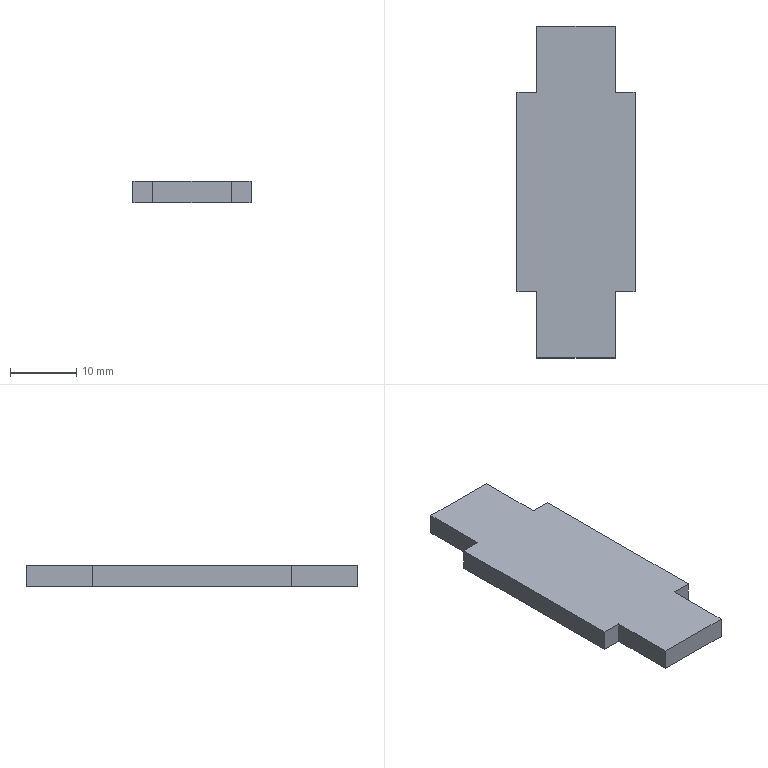Part | SolidWorks | features FlatPattern 1, SMBaseFlange 1, SheetMetal 1 | 1 solid | 14 faces | box 17.8 x 50 x 3.2 mm | volume 2464 mm3 | plane 14
STEP:
#1=CARTESIAN_POINT('',(-38.858,-170.001,0.));
#2=VERTEX_POINT('',#1);
#3=CARTESIAN_POINT('',(-38.858,-160.001,0.));
#4=VERTEX_POINT('',#3);
#5=CARTESIAN_POINT('',(-38.858,-170.001,0.));
#6=DIRECTION('',(0.,1.,0.));
#7=VECTOR('',#6,1000.);
#8=LINE('',#5,#7);
#9=EDGE_CURVE('',#2,#4,#8,.T.);
#10=ORIENTED_EDGE('',*,*,#9,.F.);
#11=CARTESIAN_POINT('',(-38.858,-170.001,-3.2));
#12=VERTEX_POINT('',#11);
#13=CARTESIAN_POINT('',(-38.858,-170.001,-3.2));
#14=DIRECTION('',(0.,0.,1.));
#15=VECTOR('',#14,1000.);
#16=LINE('',#13,#15);
#17=EDGE_CURVE('',#12,#2,#16,.T.);
#18=ORIENTED_EDGE('',*,*,#17,.F.);
#19=CARTESIAN_POINT('',(-38.858,-160.001,-3.2));
#20=VERTEX_POINT('',#19);
#21=CARTESIAN_POINT('',(-38.858,-170.001,-3.2));
#22=DIRECTION('',(0.,1.,0.));
#23=VECTOR('',#22,1000.);
#24=LINE('',#21,#23);
#25=EDGE_CURVE('',#12,#20,#24,.T.);
#26=ORIENTED_EDGE('',*,*,#25,.T.);
#27=CARTESIAN_POINT('',(-38.858,-160.001,-3.2));
#28=DIRECTION('',(0.,0.,1.));
#29=VECTOR('',#28,1000.);
#30=LINE('',#27,#29);
#31=EDGE_CURVE('',#20,#4,#30,.T.);
#32=ORIENTED_EDGE('',*,*,#31,.T.);
#33=EDGE_LOOP('',(#10,#18,#26,#32));
#34=FACE_OUTER_BOUND('',#33,.T.);
#35=CARTESIAN_POINT('',(-38.858,-170.001,-3.2));
#36=DIRECTION('',(1.,0.,0.));
#37=DIRECTION('',(0.,1.,0.));
#38=AXIS2_PLACEMENT_3D('',#35,#36,#37);
#39=PLANE('',#38);
#40=ADVANCED_FACE('',(#34),#39,.T.);
#41=CARTESIAN_POINT('',(-50.658,-170.001,0.));
#42=VERTEX_POINT('',#41);
#43=CARTESIAN_POINT('',(-38.858,-170.001,0.));
#44=DIRECTION('',(1.,0.,0.));
#45=VECTOR('',#44,1000.);
#46=LINE('',#43,#45);
#47=EDGE_CURVE('',#42,#2,#46,.T.);
#48=ORIENTED_EDGE('',*,*,#47,.F.);
#49=CARTESIAN_POINT('',(-50.658,-170.001,-3.2));
#50=VERTEX_POINT('',#49);
#51=CARTESIAN_POINT('',(-50.658,-170.001,-3.2));
#52=DIRECTION('',(0.,0.,1.));
#53=VECTOR('',#52,1000.);
#54=LINE('',#51,#53);
#55=EDGE_CURVE('',#50,#42,#54,.T.);
#56=ORIENTED_EDGE('',*,*,#55,.F.);
#57=CARTESIAN_POINT('',(-38.858,-170.001,-3.2));
#58=DIRECTION('',(1.,0.,0.));
#59=VECTOR('',#58,1000.);
#60=LINE('',#57,#59);
#61=EDGE_CURVE('',#50,#12,#60,.T.);
#62=ORIENTED_EDGE('',*,*,#61,.T.);
#63=ORIENTED_EDGE('',*,*,#17,.T.);
#64=EDGE_LOOP('',(#48,#56,#62,#63));
#65=FACE_OUTER_BOUND('',#64,.T.);
#66=CARTESIAN_POINT('',(-38.858,-170.001,-3.2));
#67=DIRECTION('',(0.,-1.,0.));
#68=DIRECTION('',(0.,0.,-1.));
#69=AXIS2_PLACEMENT_3D('',#66,#67,#68);
#70=PLANE('',#69);
#71=ADVANCED_FACE('',(#65),#70,.T.);
#72=CARTESIAN_POINT('',(-50.658,-160.001,0.));
#73=VERTEX_POINT('',#72);
#74=CARTESIAN_POINT('',(-50.658,-170.001,0.));
#75=DIRECTION('',(0.,-1.,0.));
#76=VECTOR('',#75,1000.);
#77=LINE('',#74,#76);
#78=EDGE_CURVE('',#73,#42,#77,.T.);
#79=ORIENTED_EDGE('',*,*,#78,.F.);
#80=CARTESIAN_POINT('',(-50.658,-160.001,-3.2));
#81=VERTEX_POINT('',#80);
#82=CARTESIAN_POINT('',(-50.658,-160.001,-3.2));
#83=DIRECTION('',(0.,0.,1.));
#84=VECTOR('',#83,1000.);
#85=LINE('',#82,#84);
#86=EDGE_CURVE('',#81,#73,#85,.T.);
#87=ORIENTED_EDGE('',*,*,#86,.F.);
#88=CARTESIAN_POINT('',(-50.658,-170.001,-3.2));
#89=DIRECTION('',(0.,-1.,0.));
#90=VECTOR('',#89,1000.);
#91=LINE('',#88,#90);
#92=EDGE_CURVE('',#81,#50,#91,.T.);
#93=ORIENTED_EDGE('',*,*,#92,.T.);
#94=ORIENTED_EDGE('',*,*,#55,.T.);
#95=EDGE_LOOP('',(#79,#87,#93,#94));
#96=FACE_OUTER_BOUND('',#95,.T.);
#97=CARTESIAN_POINT('',(-50.658,-170.001,-3.2));
#98=DIRECTION('',(-1.,0.,0.));
#99=DIRECTION('',(0.,0.,1.));
#100=AXIS2_PLACEMENT_3D('',#97,#98,#99);
#101=PLANE('',#100);
#102=ADVANCED_FACE('',(#96),#101,.T.);
#103=CARTESIAN_POINT('',(-53.658,-160.001,0.));
#104=VERTEX_POINT('',#103);
#105=CARTESIAN_POINT('',(-50.658,-160.001,0.));
#106=DIRECTION('',(1.,0.,0.));
#107=VECTOR('',#106,1000.);
#108=LINE('',#105,#107);
#109=EDGE_CURVE('',#104,#73,#108,.T.);
#110=ORIENTED_EDGE('',*,*,#109,.F.);
#111=CARTESIAN_POINT('',(-53.658,-160.001,-3.2));
#112=VERTEX_POINT('',#111);
#113=CARTESIAN_POINT('',(-53.658,-160.001,-3.2));
#114=DIRECTION('',(0.,0.,1.));
#115=VECTOR('',#114,1000.);
#116=LINE('',#113,#115);
#117=EDGE_CURVE('',#112,#104,#116,.T.);
#118=ORIENTED_EDGE('',*,*,#117,.F.);
#119=CARTESIAN_POINT('',(-50.658,-160.001,-3.2));
#120=DIRECTION('',(1.,0.,0.));
#121=VECTOR('',#120,1000.);
#122=LINE('',#119,#121);
#123=EDGE_CURVE('',#112,#81,#122,.T.);
#124=ORIENTED_EDGE('',*,*,#123,.T.);
#125=ORIENTED_EDGE('',*,*,#86,.T.);
#126=EDGE_LOOP('',(#110,#118,#124,#125));
#127=FACE_OUTER_BOUND('',#126,.T.);
#128=CARTESIAN_POINT('',(-50.658,-160.001,-3.2));
#129=DIRECTION('',(0.,-1.,0.));
#130=DIRECTION('',(0.,0.,-1.));
#131=AXIS2_PLACEMENT_3D('',#128,#129,#130);
#132=PLANE('',#131);
#133=ADVANCED_FACE('',(#127),#132,.T.);
#134=CARTESIAN_POINT('',(-53.658,-130.001,0.));
#135=VERTEX_POINT('',#134);
#136=CARTESIAN_POINT('',(-53.658,-160.001,0.));
#137=DIRECTION('',(0.,-1.,0.));
#138=VECTOR('',#137,1000.);
#139=LINE('',#136,#138);
#140=EDGE_CURVE('',#135,#104,#139,.T.);
#141=ORIENTED_EDGE('',*,*,#140,.F.);
#142=CARTESIAN_POINT('',(-53.658,-130.001,-3.2));
#143=VERTEX_POINT('',#142);
#144=CARTESIAN_POINT('',(-53.658,-130.001,-3.2));
#145=DIRECTION('',(0.,0.,1.));
#146=VECTOR('',#145,1000.);
#147=LINE('',#144,#146);
#148=EDGE_CURVE('',#143,#135,#147,.T.);
#149=ORIENTED_EDGE('',*,*,#148,.F.);
#150=CARTESIAN_POINT('',(-53.658,-160.001,-3.2));
#151=DIRECTION('',(0.,-1.,0.));
#152=VECTOR('',#151,1000.);
#153=LINE('',#150,#152);
#154=EDGE_CURVE('',#143,#112,#153,.T.);
#155=ORIENTED_EDGE('',*,*,#154,.T.);
#156=ORIENTED_EDGE('',*,*,#117,.T.);
#157=EDGE_LOOP('',(#141,#149,#155,#156));
#158=FACE_OUTER_BOUND('',#157,.T.);
#159=CARTESIAN_POINT('',(-53.658,-160.001,-3.2));
#160=DIRECTION('',(-1.,0.,0.));
#161=DIRECTION('',(0.,0.,1.));
#162=AXIS2_PLACEMENT_3D('',#159,#160,#161);
#163=PLANE('',#162);
#164=ADVANCED_FACE('',(#158),#163,.T.);
#165=CARTESIAN_POINT('',(-50.658,-130.001,0.));
#166=VERTEX_POINT('',#165);
#167=CARTESIAN_POINT('',(-53.658,-130.001,0.));
#168=DIRECTION('',(-1.,0.,0.));
#169=VECTOR('',#168,1000.);
#170=LINE('',#167,#169);
#171=EDGE_CURVE('',#166,#135,#170,.T.);
#172=ORIENTED_EDGE('',*,*,#171,.F.);
#173=CARTESIAN_POINT('',(-50.658,-130.001,-3.2));
#174=VERTEX_POINT('',#173);
#175=CARTESIAN_POINT('',(-50.658,-130.001,-3.2));
#176=DIRECTION('',(0.,0.,1.));
#177=VECTOR('',#176,1000.);
#178=LINE('',#175,#177);
#179=EDGE_CURVE('',#174,#166,#178,.T.);
#180=ORIENTED_EDGE('',*,*,#179,.F.);
#181=CARTESIAN_POINT('',(-53.658,-130.001,-3.2));
#182=DIRECTION('',(-1.,0.,0.));
#183=VECTOR('',#182,1000.);
#184=LINE('',#181,#183);
#185=EDGE_CURVE('',#174,#143,#184,.T.);
#186=ORIENTED_EDGE('',*,*,#185,.T.);
#187=ORIENTED_EDGE('',*,*,#148,.T.);
#188=EDGE_LOOP('',(#172,#180,#186,#187));
#189=FACE_OUTER_BOUND('',#188,.T.);
#190=CARTESIAN_POINT('',(-53.658,-130.001,-3.2));
#191=DIRECTION('',(0.,1.,0.));
#192=DIRECTION('',(0.,0.,1.));
#193=AXIS2_PLACEMENT_3D('',#190,#191,#192);
#194=PLANE('',#193);
#195=ADVANCED_FACE('',(#189),#194,.T.);
#196=CARTESIAN_POINT('',(-50.658,-120.001,0.));
#197=VERTEX_POINT('',#196);
#198=CARTESIAN_POINT('',(-50.658,-130.001,0.));
#199=DIRECTION('',(0.,-1.,0.));
#200=VECTOR('',#199,1000.);
#201=LINE('',#198,#200);
#202=EDGE_CURVE('',#197,#166,#201,.T.);
#203=ORIENTED_EDGE('',*,*,#202,.F.);
#204=CARTESIAN_POINT('',(-50.658,-120.001,-3.2));
#205=VERTEX_POINT('',#204);
#206=CARTESIAN_POINT('',(-50.658,-120.001,-3.2));
#207=DIRECTION('',(0.,0.,1.));
#208=VECTOR('',#207,1000.);
#209=LINE('',#206,#208);
#210=EDGE_CURVE('',#205,#197,#209,.T.);
#211=ORIENTED_EDGE('',*,*,#210,.F.);
#212=CARTESIAN_POINT('',(-50.658,-130.001,-3.2));
#213=DIRECTION('',(0.,-1.,0.));
#214=VECTOR('',#213,1000.);
#215=LINE('',#212,#214);
#216=EDGE_CURVE('',#205,#174,#215,.T.);
#217=ORIENTED_EDGE('',*,*,#216,.T.);
#218=ORIENTED_EDGE('',*,*,#179,.T.);
#219=EDGE_LOOP('',(#203,#211,#217,#218));
#220=FACE_OUTER_BOUND('',#219,.T.);
#221=CARTESIAN_POINT('',(-50.658,-130.001,-3.2));
#222=DIRECTION('',(-1.,0.,0.));
#223=DIRECTION('',(0.,-1.,0.));
#224=AXIS2_PLACEMENT_3D('',#221,#222,#223);
#225=PLANE('',#224);
#226=ADVANCED_FACE('',(#220),#225,.T.);
#227=CARTESIAN_POINT('',(-38.858,-120.001,0.));
#228=VERTEX_POINT('',#227);
#229=CARTESIAN_POINT('',(-38.858,-120.001,0.));
#230=DIRECTION('',(-1.,0.,0.));
#231=VECTOR('',#230,1000.);
#232=LINE('',#229,#231);
#233=EDGE_CURVE('',#228,#197,#232,.T.);
#234=ORIENTED_EDGE('',*,*,#233,.F.);
#235=CARTESIAN_POINT('',(-38.858,-120.001,-3.2));
#236=VERTEX_POINT('',#235);
#237=CARTESIAN_POINT('',(-38.858,-120.001,-3.2));
#238=DIRECTION('',(0.,0.,1.));
#239=VECTOR('',#238,1000.);
#240=LINE('',#237,#239);
#241=EDGE_CURVE('',#236,#228,#240,.T.);
#242=ORIENTED_EDGE('',*,*,#241,.F.);
#243=CARTESIAN_POINT('',(-38.858,-120.001,-3.2));
#244=DIRECTION('',(-1.,0.,0.));
#245=VECTOR('',#244,1000.);
#246=LINE('',#243,#245);
#247=EDGE_CURVE('',#236,#205,#246,.T.);
#248=ORIENTED_EDGE('',*,*,#247,.T.);
#249=ORIENTED_EDGE('',*,*,#210,.T.);
#250=EDGE_LOOP('',(#234,#242,#248,#249));
#251=FACE_OUTER_BOUND('',#250,.T.);
#252=CARTESIAN_POINT('',(-38.858,-120.001,-3.2));
#253=DIRECTION('',(0.,1.,0.));
#254=DIRECTION('',(0.,0.,1.));
#255=AXIS2_PLACEMENT_3D('',#252,#253,#254);
#256=PLANE('',#255);
#257=ADVANCED_FACE('',(#251),#256,.T.);
#258=CARTESIAN_POINT('',(-38.858,-130.001,0.));
#259=VERTEX_POINT('',#258);
#260=CARTESIAN_POINT('',(-38.858,-130.001,0.));
#261=DIRECTION('',(0.,1.,0.));
#262=VECTOR('',#261,1000.);
#263=LINE('',#260,#262);
#264=EDGE_CURVE('',#259,#228,#263,.T.);
#265=ORIENTED_EDGE('',*,*,#264,.F.);
#266=CARTESIAN_POINT('',(-38.858,-130.001,-3.2));
#267=VERTEX_POINT('',#266);
#268=CARTESIAN_POINT('',(-38.858,-130.001,-3.2));
#269=DIRECTION('',(0.,0.,1.));
#270=VECTOR('',#269,1000.);
#271=LINE('',#268,#270);
#272=EDGE_CURVE('',#267,#259,#271,.T.);
#273=ORIENTED_EDGE('',*,*,#272,.F.);
#274=CARTESIAN_POINT('',(-38.858,-130.001,-3.2));
#275=DIRECTION('',(0.,1.,0.));
#276=VECTOR('',#275,1000.);
#277=LINE('',#274,#276);
#278=EDGE_CURVE('',#267,#236,#277,.T.);
#279=ORIENTED_EDGE('',*,*,#278,.T.);
#280=ORIENTED_EDGE('',*,*,#241,.T.);
#281=EDGE_LOOP('',(#265,#273,#279,#280));
#282=FACE_OUTER_BOUND('',#281,.T.);
#283=CARTESIAN_POINT('',(-38.858,-130.001,-3.2));
#284=DIRECTION('',(1.,0.,0.));
#285=DIRECTION('',(0.,0.,-1.));
#286=AXIS2_PLACEMENT_3D('',#283,#284,#285);
#287=PLANE('',#286);
#288=ADVANCED_FACE('',(#282),#287,.T.);
#289=CARTESIAN_POINT('',(-35.858,-130.001,0.));
#290=VERTEX_POINT('',#289);
#291=CARTESIAN_POINT('',(-35.858,-130.001,0.));
#292=DIRECTION('',(-1.,0.,0.));
#293=VECTOR('',#292,1000.);
#294=LINE('',#291,#293);
#295=EDGE_CURVE('',#290,#259,#294,.T.);
#296=ORIENTED_EDGE('',*,*,#295,.F.);
#297=CARTESIAN_POINT('',(-35.858,-130.001,-3.2));
#298=VERTEX_POINT('',#297);
#299=CARTESIAN_POINT('',(-35.858,-130.001,-3.2));
#300=DIRECTION('',(0.,0.,1.));
#301=VECTOR('',#300,1000.);
#302=LINE('',#299,#301);
#303=EDGE_CURVE('',#298,#290,#302,.T.);
#304=ORIENTED_EDGE('',*,*,#303,.F.);
#305=CARTESIAN_POINT('',(-35.858,-130.001,-3.2));
#306=DIRECTION('',(-1.,0.,0.));
#307=VECTOR('',#306,1000.);
#308=LINE('',#305,#307);
#309=EDGE_CURVE('',#298,#267,#308,.T.);
#310=ORIENTED_EDGE('',*,*,#309,.T.);
#311=ORIENTED_EDGE('',*,*,#272,.T.);
#312=EDGE_LOOP('',(#296,#304,#310,#311));
#313=FACE_OUTER_BOUND('',#312,.T.);
#314=CARTESIAN_POINT('',(-35.858,-130.001,-3.2));
#315=DIRECTION('',(0.,1.,0.));
#316=DIRECTION('',(0.,0.,1.));
#317=AXIS2_PLACEMENT_3D('',#314,#315,#316);
#318=PLANE('',#317);
#319=ADVANCED_FACE('',(#313),#318,.T.);
#320=CARTESIAN_POINT('',(-35.858,-160.001,0.));
#321=VERTEX_POINT('',#320);
#322=CARTESIAN_POINT('',(-35.858,-160.001,0.));
#323=DIRECTION('',(0.,1.,0.));
#324=VECTOR('',#323,1000.);
#325=LINE('',#322,#324);
#326=EDGE_CURVE('',#321,#290,#325,.T.);
#327=ORIENTED_EDGE('',*,*,#326,.F.);
#328=CARTESIAN_POINT('',(-35.858,-160.001,-3.2));
#329=VERTEX_POINT('',#328);
#330=CARTESIAN_POINT('',(-35.858,-160.001,-3.2));
#331=DIRECTION('',(0.,0.,1.));
#332=VECTOR('',#331,1000.);
#333=LINE('',#330,#332);
#334=EDGE_CURVE('',#329,#321,#333,.T.);
#335=ORIENTED_EDGE('',*,*,#334,.F.);
#336=CARTESIAN_POINT('',(-35.858,-160.001,-3.2));
#337=DIRECTION('',(0.,1.,0.));
#338=VECTOR('',#337,1000.);
#339=LINE('',#336,#338);
#340=EDGE_CURVE('',#329,#298,#339,.T.);
#341=ORIENTED_EDGE('',*,*,#340,.T.);
#342=ORIENTED_EDGE('',*,*,#303,.T.);
#343=EDGE_LOOP('',(#327,#335,#341,#342));
#344=FACE_OUTER_BOUND('',#343,.T.);
#345=CARTESIAN_POINT('',(-35.858,-160.001,-3.2));
#346=DIRECTION('',(1.,0.,0.));
#347=DIRECTION('',(0.,0.,-1.));
#348=AXIS2_PLACEMENT_3D('',#345,#346,#347);
#349=PLANE('',#348);
#350=ADVANCED_FACE('',(#344),#349,.T.);
#351=CARTESIAN_POINT('',(-38.858,-160.001,0.));
#352=DIRECTION('',(1.,0.,0.));
#353=VECTOR('',#352,1000.);
#354=LINE('',#351,#353);
#355=EDGE_CURVE('',#4,#321,#354,.T.);
#356=ORIENTED_EDGE('',*,*,#355,.F.);
#357=ORIENTED_EDGE('',*,*,#31,.F.);
#358=CARTESIAN_POINT('',(-38.858,-160.001,-3.2));
#359=DIRECTION('',(1.,0.,0.));
#360=VECTOR('',#359,1000.);
#361=LINE('',#358,#360);
#362=EDGE_CURVE('',#20,#329,#361,.T.);
#363=ORIENTED_EDGE('',*,*,#362,.T.);
#364=ORIENTED_EDGE('',*,*,#334,.T.);
#365=EDGE_LOOP('',(#356,#357,#363,#364));
#366=FACE_OUTER_BOUND('',#365,.T.);
#367=CARTESIAN_POINT('',(-38.858,-160.001,-3.2));
#368=DIRECTION('',(0.,-1.,0.));
#369=DIRECTION('',(0.,0.,-1.));
#370=AXIS2_PLACEMENT_3D('',#367,#368,#369);
#371=PLANE('',#370);
#372=ADVANCED_FACE('',(#366),#371,.T.);
#373=ORIENTED_EDGE('',*,*,#25,.F.);
#374=ORIENTED_EDGE('',*,*,#61,.F.);
#375=ORIENTED_EDGE('',*,*,#92,.F.);
#376=ORIENTED_EDGE('',*,*,#123,.F.);
#377=ORIENTED_EDGE('',*,*,#154,.F.);
#378=ORIENTED_EDGE('',*,*,#185,.F.);
#379=ORIENTED_EDGE('',*,*,#216,.F.);
#380=ORIENTED_EDGE('',*,*,#247,.F.);
#381=ORIENTED_EDGE('',*,*,#278,.F.);
#382=ORIENTED_EDGE('',*,*,#309,.F.);
#383=ORIENTED_EDGE('',*,*,#340,.F.);
#384=ORIENTED_EDGE('',*,*,#362,.F.);
#385=EDGE_LOOP('',(#373,#374,#375,#376,#377,#378,#379,#380,#381,#382,#383,#384));
#386=FACE_OUTER_BOUND('',#385,.T.);
#387=CARTESIAN_POINT('',(0.,0.,-3.2));
#388=DIRECTION('',(0.,0.,-1.));
#389=DIRECTION('',(-1.,0.,0.));
#390=AXIS2_PLACEMENT_3D('',#387,#388,#389);
#391=PLANE('',#390);
#392=ADVANCED_FACE('',(#386),#391,.T.);
#393=ORIENTED_EDGE('',*,*,#9,.T.);
#394=ORIENTED_EDGE('',*,*,#355,.T.);
#395=ORIENTED_EDGE('',*,*,#326,.T.);
#396=ORIENTED_EDGE('',*,*,#295,.T.);
#397=ORIENTED_EDGE('',*,*,#264,.T.);
#398=ORIENTED_EDGE('',*,*,#233,.T.);
#399=ORIENTED_EDGE('',*,*,#202,.T.);
#400=ORIENTED_EDGE('',*,*,#171,.T.);
#401=ORIENTED_EDGE('',*,*,#140,.T.);
#402=ORIENTED_EDGE('',*,*,#109,.T.);
#403=ORIENTED_EDGE('',*,*,#78,.T.);
#404=ORIENTED_EDGE('',*,*,#47,.T.);
#405=EDGE_LOOP('',(#393,#394,#395,#396,#397,#398,#399,#400,#401,#402,#403,#404));
#406=FACE_OUTER_BOUND('',#405,.T.);
#407=CARTESIAN_POINT('',(0.,0.,0.));
#408=DIRECTION('',(0.,0.,-1.));
#409=DIRECTION('',(-1.,0.,0.));
#410=AXIS2_PLACEMENT_3D('',#407,#408,#409);
#411=PLANE('',#410);
#412=ADVANCED_FACE('',(#406),#411,.F.);
#413=CLOSED_SHELL('',(#40,#71,#102,#133,#164,#195,#226,#257,#288,#319,#350,#372,#392,#412));
#414=MANIFOLD_SOLID_BREP('',#413);
#415=CARTESIAN_POINT('',(0.,0.,0.));
#416=DIRECTION('',(0.,0.,1.));
#417=DIRECTION('',(1.,0.,0.));
#418=AXIS2_PLACEMENT_3D('',#415,#416,#417);
#419=(LENGTH_UNIT()NAMED_UNIT(*)SI_UNIT(.MILLI.,.METRE.));
#420=UNCERTAINTY_MEASURE_WITH_UNIT(LENGTH_MEASURE(0.00001),#419,'','');
#421=(NAMED_UNIT(*)PLANE_ANGLE_UNIT()SI_UNIT($,.RADIAN.));
#422=(NAMED_UNIT(*)SI_UNIT($,.STERADIAN.)SOLID_ANGLE_UNIT());
#423=(GEOMETRIC_REPRESENTATION_CONTEXT(3)GLOBAL_UNCERTAINTY_ASSIGNED_CONTEXT((#420))GLOBAL_UNIT_ASSIGNED_CONTEXT((#419,#421,#422))REPRESENTATION_CONTEXT('',''));
#424=ADVANCED_BREP_SHAPE_REPRESENTATION('',(#414,#418),#423);